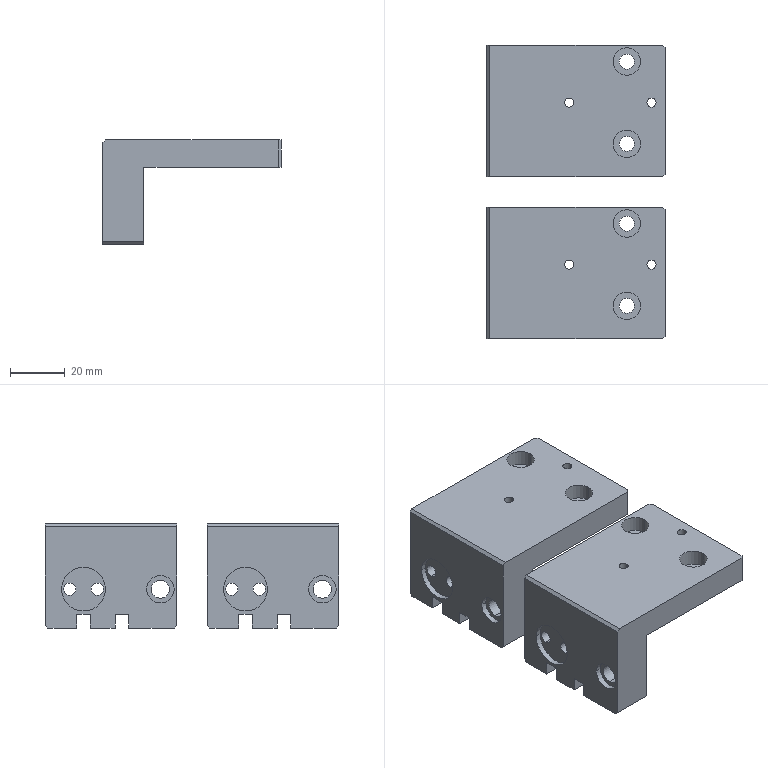NC program | NX | posted with a generic post | part box 65 x 107 x 38 mm
Whole program:
N10 G17 G21 G94 G90
(FLOOR_WALL_COPY , TOOL : D80)
N12 T19 M6
N14 G54
N16 G17 G0 G90 X96.5 Y0. B0. C0. S6500 M3
N18 G43 Z30. H19
N20 Z9.
N22 G94 G1 Z6. F1500.
N24 X93.5
N26 X-93.5
N28 X-96.5
N30 Z9.
N32 G0 Z30.
N34 X96.5
N36 Z8.
N38 G1 Z5.
N40 X93.5
N42 X-93.5
N44 X-96.5
N46 Z8.
N48 G0 Z30.
N50 X96.5
N52 Z7.
N54 G1 Z4.
N56 X93.5
N58 X-93.5
N60 X-96.5
N62 Z7.
N64 G0 Z30.
N66 X96.5
N68 Z6.
N70 G1 Z3.
N72 X93.5
N74 X-93.5
N76 X-96.5
N78 Z6.
N80 G0 Z30.
N82 X96.5
N84 Z5.
N86 G1 Z2.
N88 X93.5
N90 X-93.5
N92 X-96.5
N94 Z5.
N96 G0 Z30.
N98 X96.5
N100 Z4.
N102 G1 Z1.
N104 X93.5
N106 X-93.5
N108 X-96.5
N110 Z4.
N112 G0 Z30.
N114 X96.5
N116 Z3.
N118 G1 Z0.
N120 X93.5
N122 X-93.5
N124 X-96.5
N126 Z3.
N128 G0 Z30.
N130 M5
(FLOOR_WALL_1 , TOOL : D10)
N132 T15 M6
N134 G54
N136 G17 G0 G90 X-2.01 Y-39.324 B0. C0. S9500 M3
N138 G43 Z30. H15
N140 Z-5.925
N142 G94 G1 Z-8.925 F1000.
N144 X-3.063 Y-37.5
N146 G3 X-3.929 Y-37. R1.
N148 G1 X-55.071 F3500.
N150 X-55.57 Y-36.502
N152 X-3.43
N154 X-2.932 Y-36.003
N156 X-56.068
N158 X-56.567 Y-35.505
N160 X-2.433
N162 X-1.935 Y-35.006
N164 X-57.065
N166 X-57.563 Y-34.508
N168 X-1.437
N170 X-0.938 Y-34.009
N172 X-58.062
N174 X-58.5 Y-33.571
N176 Y-33.511
N178 X-0.5
N180 Y-33.012
N182 X-58.5
N184 Y-32.514
N186 X-0.5
N188 Y-32.015
N190 X-58.5
N192 Y-31.517
N194 X-0.5
N196 Y-31.018
N198 X-58.5
N200 Y-30.52
N202 X-0.5
N204 Y-30.021
N206 X-58.5
N208 Y-29.523
N210 X-0.5
N212 Y-29.024
N214 X-58.5
N216 Y-28.526
N218 X-0.5
N220 Y-28.027
N222 X-58.5
N224 Y-27.529
N226 X-0.5
N228 Y-27.03
N230 X-58.5
N232 Y-26.532
N234 X-0.5
N236 Y-26.033
N238 X-58.5
N240 Y-25.535
N242 X-0.5
N244 Y-25.036
N246 X-58.5
N248 Y-24.538
N250 X-0.5
N252 Y-24.039
N254 X-58.5
N256 Y-23.541
N258 X-0.5
N260 Y-23.042
N262 X-58.5
N264 Y-22.544
N266 X-0.5
N268 Y-22.045
N270 X-58.5
N272 Y-21.547
N274 X-0.5
N276 Y-21.048
N278 X-58.5
N280 Y-20.55
N282 X-0.5
N284 Y-20.052
N286 X-58.5
N288 Y-19.553
N290 X-0.5
N292 Y-19.055
N294 X-58.5
N296 Y-18.556
N298 X-0.5
N300 Y-18.058
N302 X-58.5
N304 Y-17.559
N306 X-0.5
N308 Y-17.061
N310 X-58.5
N312 Y-16.562
N314 X-0.5
N316 Y-16.064
N318 X-58.5
N320 Y-15.565
N322 X-0.5
N324 Y-15.067
N326 X-58.5
N328 Y-14.568
N330 X-0.5
N332 Y-14.07
N334 X-58.5
N336 Y-13.571
N338 X-0.5
N340 Y-13.073
N342 X-58.5
N344 Y-12.574
N346 X-0.5
N348 Y-12.076
N350 X-58.5
N352 Y-11.577
N354 X-0.5
N356 Y-11.079
N358 X-58.5
N360 Y-10.58
N362 X-0.5
N364 Y-10.082
N366 X-58.5
N368 Y-9.583
N370 X-0.5
N372 Y-9.085
N374 X-58.5
N376 Y-8.586
N378 X-0.5
N380 Y-8.088
N382 X-58.5
N384 Y-7.589
N386 X-0.5
N388 Y-7.091
N390 X-58.5
N392 Y-6.592
N394 X-0.5
N396 Y-6.094
N398 X-58.5
N400 Y-5.595
N402 X-0.5
N404 Y-5.097
N406 X-58.5
N408 Y-4.598
N410 X-0.5
N412 Y-4.1
N414 X-58.5
N416 Y-3.602
N418 X-0.5
N420 Y-3.103
N422 X-58.5
N424 Y-2.605
N426 X-0.5
N428 Y-2.106
N430 X-58.5
N432 Y-1.608
N434 X-0.5
N436 Y-1.109
N438 X-58.5
N440 Y-0.611
N442 X-0.5
N444 Y-0.112
N446 X-58.5
N448 Y0.386
N450 X-0.5
N452 Y0.885
N454 X-58.5
N456 Y1.383
N458 X-0.5
N460 Y1.882
N462 X-58.5
N464 Y2.38
N466 X-0.5
N468 Y2.879
N470 X-58.5
N472 Y3.377
N474 X-0.5
N476 Y3.876
N478 X-58.5
N480 Y4.374
N482 X-0.5
N484 Y4.873
N486 X-58.5
N488 Y5.371
N490 X-0.5
N492 Y5.87
N494 X-58.5
N496 Y6.368
N498 X-0.5
N500 Y6.867
N502 X-58.5
N504 Y7.365
N506 X-0.5
N508 Y7.864
N510 X-58.5
N512 Y8.362
N514 X-0.5
N516 Y8.861
N518 X-58.5
N520 Y9.359
N522 X-0.5
N524 Y9.858
N526 X-58.5
N528 Y10.356
N530 X-0.5
N532 Y10.855
N534 X-58.5
N536 Y11.353
N538 X-0.5
N540 Y11.852
N542 X-58.5
N544 Y12.35
N546 X-0.5
N548 Z-5.925
N550 G0 Z30.
N552 X-2.01 Y-39.324
N554 Z-24.85
N556 G1 Z-27.85 F1000.
N558 X-3.063 Y-37.5
N560 G3 X-3.929 Y-37. R1.
N562 G1 X-55.071 F3500.
N564 X-55.57 Y-36.502
N566 X-3.43
N568 X-2.932 Y-36.003
N570 X-56.068
N572 X-56.567 Y-35.505
N574 X-2.433
N576 X-1.935 Y-35.006
N578 X-57.065
N580 X-57.563 Y-34.508
N582 X-1.437
N584 X-0.938 Y-34.009
N586 X-58.062
N588 X-58.5 Y-33.571
N590 Y-33.511
N592 X-0.5
N594 Y-33.012
N596 X-58.5
N598 Y-32.514
N600 X-0.5
N602 Y-32.015
N604 X-58.5
N606 Y-31.517
N608 X-0.5
N610 Y-31.018
N612 X-58.5
N614 Y-30.52
N616 X-0.5
N618 Y-30.021
N620 X-58.5
N622 Y-29.523
N624 X-0.5
N626 Y-29.024
N628 X-58.5
N630 Y-28.526
N632 X-0.5
N634 Y-28.027
N636 X-58.5
N638 Y-27.529
N640 X-0.5
N642 Y-27.03
N644 X-58.5
N646 Y-26.532
N648 X-0.5
N650 Y-26.033
N652 X-58.5
N654 Y-25.535
N656 X-0.5
N658 Y-25.036
N660 X-58.5
N662 Y-24.538
N664 X-0.5
N666 Y-24.039
N668 X-58.5
N670 Y-23.541
N672 X-0.5
N674 Y-23.042
N676 X-58.5
N678 Y-22.544
N680 X-0.5
N682 Y-22.045
N684 X-58.5
N686 Y-21.547
N688 X-0.5
N690 Y-21.048
N692 X-58.5
N694 Y-20.55
N696 X-0.5
N698 Y-20.052
N700 X-58.5
N702 Y-19.553
N704 X-0.5
N706 Y-19.055
N708 X-58.5
N710 Y-18.556
N712 X-0.5
N714 Y-18.058
N716 X-58.5
N718 Y-17.559
N720 X-0.5
N722 Y-17.061
N724 X-58.5
N726 Y-16.562
N728 X-0.5
N730 Y-16.064
N732 X-58.5
N734 Y-15.565
N736 X-0.5
N738 Y-15.067
N740 X-58.5
N742 Y-14.568
N744 X-0.5
N746 Y-14.07
N748 X-58.5
N750 Y-13.571
N752 X-0.5
N754 Y-13.073
N756 X-58.5
N758 Y-12.574
N760 X-0.5
N762 Y-12.076
N764 X-58.5
N766 Y-11.577
N768 X-0.5
N770 Y-11.079
N772 X-58.5
N774 Y-10.58
N776 X-0.5
N778 Y-10.082
N780 X-58.5
N782 Y-9.583
N784 X-0.5
N786 Y-9.085
N788 X-58.5
N790 Y-8.586
N792 X-0.5
N794 Y-8.088
N796 X-58.5
N798 Y-7.589
N800 X-0.5
N802 Y-7.091
N804 X-58.5
N806 Y-6.592
N808 X-0.5
N810 Y-6.094
N812 X-58.5
N814 Y-5.595
N816 X-0.5
N818 Y-5.097
N820 X-58.5
N822 Y-4.598
N824 X-0.5
N826 Y-4.1
N828 X-58.5
N830 Y-3.602
N832 X-0.5
N834 Y-3.103
N836 X-58.5
N838 Y-2.605
N840 X-0.5
N842 Y-2.106
N844 X-58.5
N846 Y-1.608
N848 X-0.5
N850 Y-1.109
N852 X-58.5
N854 Y-0.611
N856 X-0.5
N858 Y-0.112
N860 X-58.5
N862 Y0.386
N864 X-0.5
N866 Y0.885
N868 X-58.5
N870 Y1.383
N872 X-0.5
N874 Y1.882
N876 X-58.5
N878 Y2.38
N880 X-0.5
N882 Y2.879
N884 X-58.5
N886 Y3.377
N888 X-0.5
N890 Y3.876
N892 X-58.5
N894 Y4.374
N896 X-0.5
N898 Y4.873
N900 X-58.5
N902 Y5.371
N904 X-0.5
N906 Y5.87
N908 X-58.5
N910 Y6.368
N912 X-0.5
N914 Y6.867
N916 X-58.5
N918 Y7.365
N920 X-0.5
N922 Y7.864
N924 X-58.5
N926 Y8.362
N928 X-0.5
N930 Y8.861
N932 X-58.5
N934 Y9.359
N936 X-0.5
N938 Y9.858
N940 X-58.5
N942 Y10.356
N944 X-0.5
N946 Y10.855
N948 X-58.5
N950 Y11.353
N952 X-0.5
N954 Y11.852
N956 X-58.5
N958 Y12.35
N960 X-0.5
N962 Z-24.85
N964 G0 Z30.
N966 X56.99 Y-39.324
N968 Z-5.925
N970 G1 Z-8.925 F1000.
N972 X55.937 Y-37.5
N974 G3 X55.071 Y-37. R1.
N976 G1 X3.929 F3500.
N978 X3.43 Y-36.502
N980 X55.57
N982 X56.068 Y-36.003
N984 X2.932
N986 X2.433 Y-35.505
N988 X56.567
N990 X57.065 Y-35.006
N992 X1.935
N994 X1.437 Y-34.508
N996 X57.563
N998 X58.062 Y-34.009
N1000 X0.938
N1002 X0.5 Y-33.571
N1004 Y-33.511
N1006 X58.5
N1008 Y-33.012
N1010 X0.5
N1012 Y-32.514
N1014 X58.5
N1016 Y-32.015
N1018 X0.5
N1020 Y-31.517
N1022 X58.5
N1024 Y-31.018
N1026 X0.5
N1028 Y-30.52
N1030 X58.5
N1032 Y-30.021
N1034 X0.5
N1036 Y-29.523
N1038 X58.5
N1040 Y-29.024
N1042 X0.5
N1044 Y-28.526
N1046 X58.5
N1048 Y-28.027
N1050 X0.5
N1052 Y-27.529
N1054 X58.5
N1056 Y-27.03
N1058 X0.5
N1060 Y-26.532
N1062 X58.5
N1064 Y-26.033
N1066 X0.5
N1068 Y-25.535
N1070 X58.5
N1072 Y-25.036
N1074 X0.5
N1076 Y-24.538
N1078 X58.5
N1080 Y-24.039
N1082 X0.5
N1084 Y-23.541
N1086 X58.5
N1088 Y-23.042
N1090 X0.5
N1092 Y-22.544
N1094 X58.5
N1096 Y-22.045
N1098 X0.5
N1100 Y-21.547
N1102 X58.5
N1104 Y-21.048
N1106 X0.5
N1108 Y-20.55
N1110 X58.5
N1112 Y-20.052
N1114 X0.5
N1116 Y-19.553
N1118 X58.5
N1120 Y-19.055
N1122 X0.5
N1124 Y-18.556
N1126 X58.5
N1128 Y-18.058
N1130 X0.5
N1132 Y-17.559
N1134 X58.5
N1136 Y-17.061
N1138 X0.5
N1140 Y-16.562
N1142 X58.5
N1144 Y-16.064
N1146 X0.5
N1148 Y-15.565
N1150 X58.5
N1152 Y-15.067
N1154 X0.5
N1156 Y-14.568
N1158 X58.5
N1160 Y-14.07
N1162 X0.5
N1164 Y-13.571
N1166 X58.5
N1168 Y-13.073
N1170 X0.5
N1172 Y-12.574
N1174 X58.5
N1176 Y-12.076
N1178 X0.5
N1180 Y-11.577
N1182 X58.5
N1184 Y-11.079
N1186 X0.5
N1188 Y-10.58
N1190 X58.5
N1192 Y-10.082
N1194 X0.5
N1196 Y-9.583
N1198 X58.5
N1200 Y-9.085
N1202 X0.5
N1204 Y-8.586
N1206 X58.5
N1208 Y-8.088
N1210 X0.5
N1212 Y-7.589
N1214 X58.5
N1216 Y-7.091
N1218 X0.5
N1220 Y-6.592
N1222 X58.5
N1224 Y-6.094
N1226 X0.5
N1228 Y-5.595
N1230 X58.5
N1232 Y-5.097
N1234 X0.5
N1236 Y-4.598
N1238 X58.5
N1240 Y-4.1
N1242 X0.5
N1244 Y-3.602
N1246 X58.5
N1248 Y-3.103
N1250 X0.5
N1252 Y-2.605
N1254 X58.5
N1256 Y-2.106
N1258 X0.5
N1260 Y-1.608
N1262 X58.5
N1264 Y-1.109
N1266 X0.5
N1268 Y-0.611
N1270 X58.5
N1272 Y-0.112
N1274 X0.5
N1276 Y0.386
N1278 X58.5
N1280 Y0.885
N1282 X0.5
N1284 Y1.383
N1286 X58.5
N1288 Y1.882
N1290 X0.5
N1292 Y2.38
N1294 X58.5
N1296 Y2.879
N1298 X0.5
N1300 Y3.377
N1302 X58.5
N1304 Y3.876
N1306 X0.5
N1308 Y4.374
N1310 X58.5
N1312 Y4.873
N1314 X0.5
N1316 Y5.371
N1318 X58.5
N1320 Y5.87
N1322 X0.5
N1324 Y6.368
N1326 X58.5
N1328 Y6.867
N1330 X0.5
N1332 Y7.365
N1334 X58.5
N1336 Y7.864
N1338 X0.5
N1340 Y8.362
N1342 X58.5
N1344 Y8.861
N1346 X0.5
N1348 Y9.359
N1350 X58.5
N1352 Y9.858
N1354 X0.5
N1356 Y10.356
N1358 X58.5
N1360 Y10.855
N1362 X0.5
N1364 Y11.353
N1366 X58.5
N1368 Y11.852
N1370 X0.5
N1372 Y12.35
N1374 X58.5
N1376 G2 X59.366 Y11.85 R1.
N1378 G1 X61.5 Y8.154
N1380 Z-5.925
N1382 G0 Z30.
N1384 X56.99 Y-39.324
N1386 Z-24.85
N1388 G1 Z-27.85 F1000.
N1390 X55.937 Y-37.5
N1392 G3 X55.071 Y-37. R1.
N1394 G1 X3.929 F3500.
N1396 X3.43 Y-36.502
N1398 X55.57
N1400 X56.068 Y-36.003
N1402 X2.932
N1404 X2.433 Y-35.505
N1406 X56.567
N1408 X57.065 Y-35.006
N1410 X1.935
N1412 X1.437 Y-34.508
N1414 X57.563
N1416 X58.062 Y-34.009
N1418 X0.938
N1420 X0.5 Y-33.571
N1422 Y-33.511
N1424 X58.5
N1426 Y-33.012
N1428 X0.5
N1430 Y-32.514
N1432 X58.5
N1434 Y-32.015
N1436 X0.5
N1438 Y-31.517
N1440 X58.5
N1442 Y-31.018
N1444 X0.5
N1446 Y-30.52
N1448 X58.5
N1450 Y-30.021
N1452 X0.5
N1454 Y-29.523
N1456 X58.5
N1458 Y-29.024
N1460 X0.5
N1462 Y-28.526
N1464 X58.5
N1466 Y-28.027
N1468 X0.5
N1470 Y-27.529
N1472 X58.5
N1474 Y-27.03
N1476 X0.5
N1478 Y-26.532
N1480 X58.5
N1482 Y-26.033
N1484 X0.5
N1486 Y-25.535
N1488 X58.5
N1490 Y-25.036
N1492 X0.5
N1494 Y-24.538
N1496 X58.5
N1498 Y-24.039
N1500 X0.5
N1502 Y-23.541
N1504 X58.5
N1506 Y-23.042
N1508 X0.5
N1510 Y-22.544
N1512 X58.5
N1514 Y-22.045
N1516 X0.5
N1518 Y-21.547
N1520 X58.5
N1522 Y-21.048
N1524 X0.5
N1526 Y-20.55
N1528 X58.5
N1530 Y-20.052
N1532 X0.5
N1534 Y-19.553
N1536 X58.5
N1538 Y-19.055
N1540 X0.5
N1542 Y-18.556
N1544 X58.5
N1546 Y-18.058
N1548 X0.5
N1550 Y-17.559
N1552 X58.5
N1554 Y-17.061
N1556 X0.5
N1558 Y-16.562
N1560 X58.5
N1562 Y-16.064
N1564 X0.5
N1566 Y-15.565
N1568 X58.5
N1570 Y-15.067
N1572 X0.5
N1574 Y-14.568
N1576 X58.5
N1578 Y-14.07
N1580 X0.5
N1582 Y-13.571
N1584 X58.5
N1586 Y-13.073
N1588 X0.5
N1590 Y-12.574
N1592 X58.5
N1594 Y-12.076
N1596 X0.5
N1598 Y-11.577
N1600 X58.5
N1602 Y-11.079
N1604 X0.5
N1606 Y-10.58
N1608 X58.5
N1610 Y-10.082
N1612 X0.5
N1614 Y-9.583
N1616 X58.5
N1618 Y-9.085
N1620 X0.5
N1622 Y-8.586
N1624 X58.5
N1626 Y-8.088
N1628 X0.5
N1630 Y-7.589
N1632 X58.5
N1634 Y-7.091
N1636 X0.5
N1638 Y-6.592
N1640 X58.5
N1642 Y-6.094
N1644 X0.5
N1646 Y-5.595
N1648 X58.5
N1650 Y-5.097
N1652 X0.5
N1654 Y-4.598
N1656 X58.5
N1658 Y-4.1
N1660 X0.5
N1662 Y-3.602
N1664 X58.5
N1666 Y-3.103
N1668 X0.5
N1670 Y-2.605
N1672 X58.5
N1674 Y-2.106
N1676 X0.5
N1678 Y-1.608
N1680 X58.5
N1682 Y-1.109
N1684 X0.5
N1686 Y-0.611
N1688 X58.5
N1690 Y-0.112
N1692 X0.5
N1694 Y0.386
N1696 X58.5
N1698 Y0.885
N1700 X0.5
N1702 Y1.383
N1704 X58.5
N1706 Y1.882
N1708 X0.5
N1710 Y2.38
N1712 X58.5
N1714 Y2.879
N1716 X0.5
N1718 Y3.377
N1720 X58.5
N1722 Y3.876
N1724 X0.5
N1726 Y4.374
N1728 X58.5
N1730 Y4.873
N1732 X0.5
N1734 Y5.371
N1736 X58.5
N1738 Y5.87
N1740 X0.5
N1742 Y6.368
N1744 X58.5
N1746 Y6.867
N1748 X0.5
N1750 Y7.365
N1752 X58.5
N1754 Y7.864
N1756 X0.5
N1758 Y8.362
N1760 X58.5
N1762 Y8.861
N1764 X0.5
N1766 Y9.359
N1768 X58.5
N1770 Y9.858
N1772 X0.5
N1774 Y10.356
N1776 X58.5
N1778 Y10.855
N1780 X0.5
N1782 Y11.353
N1784 X58.5
N1786 Y11.852
N1788 X0.5
N1790 Y12.35
N1792 X58.5
N1794 G2 X59.366 Y11.85 R1.
N1796 G1 X61.5 Y8.154
N1798 Z-24.85
N1800 G0 Z30.
N1802 M5
(FLOOR_WALL_2 , TOOL : D10JING)
N1804 T14 M6
N1806 G54
N1808 G17 G0 G90 X-61.65 Y11.847 B0. C0. S9500 M3
N1810 G43 Z30. H14
N1812 Z-25.
N1814 G94 G1 Z-28. F1500.
N1816 X-58.5
N1818 X-0.5
N1820 Y7.364
N1822 X-58.5
N1824 Y2.881
N1826 X-0.5
N1828 Y-1.602
N1830 X-58.5
N1832 Y-6.085
N1834 X-0.5
N1836 Y-10.568
N1838 X-58.5
N1840 Y-15.051
N1842 X-0.5
N1844 Y-19.534
N1846 X-58.5
N1848 Y-24.017
N1850 X-0.5
N1852 Y-28.5
N1854 X-58.5
N1856 X-61.5
N1858 Z-25.
N1860 G0 Z30.
N1862 X-0.5 Y-10.042
N1864 Z-22.
N1866 G1 Y12.35 Z-28.
N1868 X-58.5
N1870 X-61.65
N1872 Z-25.
N1874 G0 Z30.
N1876 X61.5 Y-32.497
N1878 Z-25.
N1880 G1 Z-28.
N1882 X58.5
N1884 X0.5
N1886 Y-27.57
N1888 X58.5
N1890 Y-22.642
N1892 X0.5
N1894 Y-17.715
N1896 X58.5
N1898 Y-12.787
N1900 X0.5
N1902 Y-7.86
N1904 X58.5
N1906 Y-2.932
N1908 X0.5
N1910 Y1.995
N1912 X58.5
N1914 Y6.923
N1916 X0.5
N1918 Y11.85
N1920 X58.5
N1922 X61.65
N1924 Z-25.
N1926 G0 Z30.
N1928 Y12.35
N1930 Z-25.
N1932 G1 Z-28.
N1934 X58.5
N1936 X0.5
N1938 X-2.5
N1940 Y9.35
N1942 Z-25.
N1944 G0 Z30.
(FLOOR_WALL_2_COPY , TOOL : D10JING)
N1946 X-3.191 Y9.5
N1948 Z-6.
N1950 G1 Z-9.
N1952 X-4.634 Y12.
N1954 G3 X-5.5 Y12.5 R1.
N1956 G1 X-53.5
N1958 G3 X-54.366 Y12. R1.
N1960 G1 X-55.809 Y9.5
N1962 Z-6.
N1964 G0 Z30.
N1966 X-3.191
N1968 Z-25.
N1970 G1 Z-28.
N1972 X-4.634 Y12.
N1974 G3 X-5.5 Y12.5 R1.
N1976 G1 X-53.5
N1978 G3 X-54.366 Y12. R1.
N1980 G1 X-55.809 Y9.5
N1982 Z-25.
N1984 G0 Z30.
N1986 X55.809
N1988 Z-6.
N1990 G1 Z-9.
N1992 X54.366 Y12.
N1994 G3 X53.5 Y12.5 R1.
N1996 G1 X5.5
N1998 G3 X4.634 Y12. R1.
N2000 G1 X3.191 Y9.5
N2002 Z-6.
N2004 G0 Z30.
N2006 X55.809
N2008 Z-25.
N2010 G1 Z-28.
N2012 X54.366 Y12.
N2014 G3 X53.5 Y12.5 R1.
N2016 G1 X5.5
N2018 G3 X4.634 Y12. R1.
N2020 G1 X3.191 Y9.5
N2022 Z-25.
N2024 G0 Z30.
N2026 M5
(FLOOR_WALL_3 , TOOL : D4)
N2028 T11 M6
N2030 G54
N2032 G17 G0 G90 X-39.5 Y37.5 B0. C0. S9500 M3
N2034 G43 Z30. H11
N2036 Z2.615
N2038 G94 G1 Z-0.385 F1500.
N2040 Y32.5
N2042 X-39.
N2044 Y17.5
N2046 X-40.
N2048 Y32.5
N2050 X-39.5
N2052 Y37.5
N2054 Z2.615
N2056 G0 Z2.231
N2058 G1 Z-0.769
N2060 Y32.5
N2062 X-39.
N2064 Y17.5
N2066 X-40.
N2068 Y32.5
N2070 X-39.5
N2072 Y37.5
N2074 Z2.231
N2076 G0 Z1.846
N2078 G1 Z-1.154
N2080 Y32.5
N2082 X-39.
N2084 Y17.5
N2086 X-40.
N2088 Y32.5
N2090 X-39.5
N2092 Y37.5
N2094 Z1.846
N2096 G0 Z1.462
N2098 G1 Z-1.538
N2100 Y32.5
N2102 X-39.
N2104 Y17.5
N2106 X-40.
N2108 Y32.5
N2110 X-39.5
N2112 Y37.5
N2114 Z1.462
N2116 G0 Z1.077
N2118 G1 Z-1.923
N2120 Y32.5
N2122 X-39.
N2124 Y17.5
N2126 X-40.
N2128 Y32.5
N2130 X-39.5
N2132 Y37.5
N2134 Z1.077
N2136 G0 Z0.692
N2138 G1 Z-2.308
N2140 Y32.5
N2142 X-39.
N2144 Y17.5
N2146 X-40.
N2148 Y32.5
N2150 X-39.5
N2152 Y37.5
N2154 Z0.692
N2156 G0 Z0.308
N2158 G1 Z-2.692
N2160 Y32.5
N2162 X-39.
N2164 Y17.5
N2166 X-40.
N2168 Y32.5
N2170 X-39.5
N2172 Y37.5
N2174 Z0.308
N2176 G0 Z-0.077
N2178 G1 Z-3.077
N2180 Y32.5
N2182 X-39.
N2184 Y17.5
N2186 X-40.
N2188 Y32.5
N2190 X-39.5
N2192 Y37.5
N2194 Z-0.077
N2196 G0 Z-0.462
N2198 G1 Z-3.462
N2200 Y32.5
N2202 X-39.
N2204 Y17.5
N2206 X-40.
N2208 Y32.5
N2210 X-39.5
N2212 Y37.5
N2214 Z-0.462
N2216 G0 Z-0.846
N2218 G1 Z-3.846
N2220 Y32.5
N2222 X-39.
N2224 Y17.5
N2226 X-40.
N2228 Y32.5
N2230 X-39.5
N2232 Y37.5
N2234 Z-0.846
N2236 G0 Z-1.231
N2238 G1 Z-4.231
N2240 Y32.5
N2242 X-39.
N2244 Y17.5
N2246 X-40.
N2248 Y32.5
N2250 X-39.5
N2252 Y37.5
N2254 Z-1.231
N2256 G0 Z-1.615
N2258 G1 Z-4.615
N2260 Y32.5
N2262 X-39.
N2264 Y17.5
N2266 X-40.
N2268 Y32.5
N2270 X-39.5
N2272 Y37.5
N2274 Z-1.615
N2276 G0 Z-2.
N2278 G1 Z-5.
N2280 Y32.5
N2282 X-39.
N2284 Y17.5
N2286 X-40.
N2288 Y32.5
N2290 X-39.5
N2292 Y37.5
N2294 Z-2.
N2296 G0 Z30.
N2298 X-25.5
N2300 Z2.615
N2302 G1 Z-0.385
N2304 Y32.5
N2306 X-25.
N2308 Y17.5
N2310 X-26.
N2312 Y32.5
N2314 X-25.5
N2316 Y37.5
N2318 Z2.615
N2320 G0 Z2.231
N2322 G1 Z-0.769
N2324 Y32.5
N2326 X-25.
N2328 Y17.5
N2330 X-26.
N2332 Y32.5
N2334 X-25.5
N2336 Y37.5
N2338 Z2.231
N2340 G0 Z1.846
N2342 G1 Z-1.154
N2344 Y32.5
N2346 X-25.
N2348 Y17.5
N2350 X-26.
N2352 Y32.5
N2354 X-25.5
N2356 Y37.5
N2358 Z1.846
N2360 G0 Z1.462
N2362 G1 Z-1.538
N2364 Y32.5
N2366 X-25.
N2368 Y17.5
N2370 X-26.
N2372 Y32.5
N2374 X-25.5
N2376 Y37.5
N2378 Z1.462
N2380 G0 Z1.077
N2382 G1 Z-1.923
N2384 Y32.5
N2386 X-25.
N2388 Y17.5
N2390 X-26.
N2392 Y32.5
N2394 X-25.5
N2396 Y37.5
N2398 Z1.077
N2400 G0 Z0.692
N2402 G1 Z-2.308
N2404 Y32.5
N2406 X-25.
N2408 Y17.5
N2410 X-26.
N2412 Y32.5
N2414 X-25.5
N2416 Y37.5
N2418 Z0.692
N2420 G0 Z0.308
N2422 G1 Z-2.692
N2424 Y32.5
N2426 X-25.
N2428 Y17.5
N2430 X-26.
N2432 Y32.5
N2434 X-25.5
N2436 Y37.5
N2438 Z0.308
N2440 G0 Z-0.077
N2442 G1 Z-3.077
N2444 Y32.5
N2446 X-25.
N2448 Y17.5
N2450 X-26.
N2452 Y32.5
N2454 X-25.5
N2456 Y37.5
N2458 Z-0.077
N2460 G0 Z-0.462
N2462 G1 Z-3.462
N2464 Y32.5
N2466 X-25.
N2468 Y17.5
N2470 X-26.
N2472 Y32.5
N2474 X-25.5
N2476 Y37.5
N2478 Z-0.462
N2480 G0 Z-0.846
N2482 G1 Z-3.846
N2484 Y32.5
N2486 X-25.
N2488 Y17.5
N2490 X-26.
N2492 Y32.5
N2494 X-25.5
N2496 Y37.5
N2498 Z-0.846
N2500 G0 Z-1.231
N2502 G1 Z-4.231
N2504 Y32.5
N2506 X-25.
N2508 Y17.5
N2510 X-26.
N2512 Y32.5
N2514 X-25.5
N2516 Y37.5
N2518 Z-1.231
N2520 G0 Z-1.615
N2522 G1 Z-4.615
N2524 Y32.5
N2526 X-25.
N2528 Y17.5
N2530 X-26.
N2532 Y32.5
N2534 X-25.5
N2536 Y37.5
N2538 Z-1.615
N2540 G0 Z-2.
N2542 G1 Z-5.
N2544 Y32.5
N2546 X-25.
N2548 Y17.5
N2550 X-26.
N2552 Y32.5
N2554 X-25.5
N2556 Y37.5
N2558 Z-2.
N2560 G0 Z30.
N2562 X19.5
N2564 Z2.615
N2566 G1 Z-0.385
N2568 Y32.5
N2570 X20.
N2572 Y17.5
N2574 X19.
N2576 Y32.5
N2578 X19.5
N2580 Y37.5
N2582 Z2.615
N2584 G0 Z2.231
N2586 G1 Z-0.769
N2588 Y32.5
N2590 X20.
N2592 Y17.5
N2594 X19.
N2596 Y32.5
N2598 X19.5
N2600 Y37.5
N2602 Z2.231
N2604 G0 Z1.846
N2606 G1 Z-1.154
N2608 Y32.5
N2610 X20.
N2612 Y17.5
N2614 X19.
N2616 Y32.5
N2618 X19.5
N2620 Y37.5
N2622 Z1.846
N2624 G0 Z1.462
N2626 G1 Z-1.538
N2628 Y32.5
N2630 X20.
N2632 Y17.5
N2634 X19.
N2636 Y32.5
N2638 X19.5
N2640 Y37.5
N2642 Z1.462
N2644 G0 Z1.077
N2646 G1 Z-1.923
N2648 Y32.5
N2650 X20.
N2652 Y17.5
N2654 X19.
N2656 Y32.5
N2658 X19.5
N2660 Y37.5
N2662 Z1.077
N2664 G0 Z0.692
N2666 G1 Z-2.308
N2668 Y32.5
N2670 X20.
N2672 Y17.5
N2674 X19.
N2676 Y32.5
N2678 X19.5
N2680 Y37.5
N2682 Z0.692
N2684 G0 Z0.308
N2686 G1 Z-2.692
N2688 Y32.5
N2690 X20.
N2692 Y17.5
N2694 X19.
N2696 Y32.5
N2698 X19.5
N2700 Y37.5
N2702 Z0.308
N2704 G0 Z-0.077
N2706 G1 Z-3.077
N2708 Y32.5
N2710 X20.
N2712 Y17.5
N2714 X19.
N2716 Y32.5
N2718 X19.5
N2720 Y37.5
N2722 Z-0.077
N2724 G0 Z-0.462
N2726 G1 Z-3.462
N2728 Y32.5
N2730 X20.
N2732 Y17.5
N2734 X19.
N2736 Y32.5
N2738 X19.5
N2740 Y37.5
N2742 Z-0.462
N2744 G0 Z-0.846
N2746 G1 Z-3.846
N2748 Y32.5
N2750 X20.
N2752 Y17.5
N2754 X19.
N2756 Y32.5
N2758 X19.5
N2760 Y37.5
N2762 Z-0.846
N2764 G0 Z-1.231
N2766 G1 Z-4.231
N2768 Y32.5
N2770 X20.
N2772 Y17.5
N2774 X19.
N2776 Y32.5
N2778 X19.5
N2780 Y37.5
N2782 Z-1.231
N2784 G0 Z-1.615
N2786 G1 Z-4.615
N2788 Y32.5
N2790 X20.
N2792 Y17.5
N2794 X19.
N2796 Y32.5
N2798 X19.5
N2800 Y37.5
N2802 Z-1.615
N2804 G0 Z-2.
N2806 G1 Z-5.
N2808 Y32.5
N2810 X20.
N2812 Y17.5
N2814 X19.
N2816 Y32.5
N2818 X19.5
N2820 Y37.5
N2822 Z-2.
N2824 G0 Z30.
N2826 X33.5
N2828 Z2.615
N2830 G1 Z-0.385
N2832 Y32.5
N2834 X34.
N2836 Y17.5
N2838 X33.
N2840 Y32.5
N2842 X33.5
N2844 Y37.5
N2846 Z2.615
N2848 G0 Z2.231
N2850 G1 Z-0.769
N2852 Y32.5
N2854 X34.
N2856 Y17.5
N2858 X33.
N2860 Y32.5
N2862 X33.5
N2864 Y37.5
N2866 Z2.231
N2868 G0 Z1.846
N2870 G1 Z-1.154
N2872 Y32.5
N2874 X34.
N2876 Y17.5
N2878 X33.
N2880 Y32.5
N2882 X33.5
N2884 Y37.5
N2886 Z1.846
N2888 G0 Z1.462
N2890 G1 Z-1.538
N2892 Y32.5
N2894 X34.
N2896 Y17.5
N2898 X33.
N2900 Y32.5
N2902 X33.5
N2904 Y37.5
N2906 Z1.462
N2908 G0 Z1.077
N2910 G1 Z-1.923
N2912 Y32.5
N2914 X34.
N2916 Y17.5
N2918 X33.
N2920 Y32.5
N2922 X33.5
N2924 Y37.5
N2926 Z1.077
N2928 G0 Z0.692
N2930 G1 Z-2.308
N2932 Y32.5
N2934 X34.
N2936 Y17.5
N2938 X33.
N2940 Y32.5
N2942 X33.5
N2944 Y37.5
N2946 Z0.692
N2948 G0 Z0.308
N2950 G1 Z-2.692
N2952 Y32.5
N2954 X34.
N2956 Y17.5
N2958 X33.
N2960 Y32.5
N2962 X33.5
N2964 Y37.5
N2966 Z0.308
N2968 G0 Z-0.077
N2970 G1 Z-3.077
N2972 Y32.5
N2974 X34.
N2976 Y17.5
N2978 X33.
N2980 Y32.5
N2982 X33.5
N2984 Y37.5
N2986 Z-0.077
N2988 G0 Z-0.462
N2990 G1 Z-3.462
N2992 Y32.5
N2994 X34.
N2996 Y17.5
N2998 X33.
N3000 Y32.5
N3002 X33.5
N3004 Y37.5
N3006 Z-0.462
N3008 G0 Z-0.846
N3010 G1 Z-3.846
N3012 Y32.5
N3014 X34.
N3016 Y17.5
N3018 X33.
N3020 Y32.5
N3022 X33.5
N3024 Y37.5
N3026 Z-0.846
N3028 G0 Z-1.231
N3030 G1 Z-4.231
N3032 Y32.5
N3034 X34.
N3036 Y17.5
N3038 X33.
N3040 Y32.5
N3042 X33.5
N3044 Y37.5
N3046 Z-1.231
N3048 G0 Z-1.615
N3050 G1 Z-4.615
N3052 Y32.5
N3054 X34.
N3056 Y17.5
N3058 X33.
N3060 Y32.5
N3062 X33.5
N3064 Y37.5
N3066 Z-1.615
N3068 G0 Z-2.
N3070 G1 Z-5.
N3072 Y32.5
N3074 X34.
N3076 Y17.5
N3078 X33.
N3080 Y32.5
N3082 X33.5
N3084 Y37.5
N3086 Z-2.
N3088 G0 Z30.
N3090 M5
(PLANAR_MILL_COPY_COPY_COPY_COPY , TOOL : D6A45)
N3092 T01 M6
N3094 G54
N3096 G17 G0 G90 X45.616 Y16.1 B0. C0. S9500 M3
N3098 G43 Z30. H1
N3100 Z0.5
N3102 G94 G1 Z-1. F1250.
N3104 G3 X44.75 Y16.6 R1.
N3106 G1 X36.
N3108 G2 X35.1 Y17.5 R0.9
N3110 G1 Y32.5
N3112 G2 X36. Y33.4 R0.9
N3114 G1 X53.5
N3116 G2 X54.4 Y32.5 R0.9
N3118 G1 Y17.5
N3120 G2 X53.5 Y16.6 R0.9
N3122 G1 X44.75
N3124 G3 X43.884 Y16.1 R1.
N3126 G1 Z0.5
N3128 G0 Z30.
N3130 X32.4 Y25.866
N3132 Z0.5
N3134 G1 Z-1.
N3136 G3 X31.9 Y25. R1.
N3138 G1 Y17.5
N3140 G2 X31. Y16.6 R0.9
N3142 G1 X22.
N3144 G2 X21.1 Y17.5 R0.9
N3146 G1 Y32.5
N3148 G2 X22. Y33.4 R0.9
N3150 G1 X31.
N3152 G2 X31.9 Y32.5 R0.9
N3154 G1 Y25.
N3156 G3 X32.4 Y24.134 R1.
N3158 G1 Z0.5
N3160 G0 Z30.
N3162 X18.4 Y25.866
N3164 Z0.5
N3166 G1 Z-1.
N3168 G3 X17.9 Y25. R1.
N3170 G1 Y17.5
N3172 G2 X17. Y16.6 R0.9
N3174 G1 X5.5
N3176 G2 X4.6 Y17.5 R0.9
N3178 G1 Y32.5
N3180 G2 X5.5 Y33.4 R0.9
N3182 G1 X17.
N3184 G2 X17.9 Y32.5 R0.9
N3186 G1 Y25.
N3188 G3 X18.4 Y24.134 R1.
N3190 G1 Z0.5
N3192 G0 Z30.
N3194 X-13.384 Y16.1
N3196 Z0.5
N3198 G1 Z-1.
N3200 G3 X-14.25 Y16.6 R1.
N3202 G1 X-23.
N3204 G2 X-23.9 Y17.5 R0.9
N3206 G1 Y32.5
N3208 G2 X-23. Y33.4 R0.9
N3210 G1 X-5.5
N3212 G2 X-4.6 Y32.5 R0.9
N3214 G1 Y17.5
N3216 G2 X-5.5 Y16.6 R0.9
N3218 G1 X-14.25
N3220 G3 X-15.116 Y16.1 R1.
N3222 G1 Z0.5
N3224 G0 Z30.
N3226 X-26.6 Y25.866
N3228 Z0.5
N3230 G1 Z-1.
N3232 G3 X-27.1 Y25. R1.
N3234 G1 Y17.5
N3236 G2 X-28. Y16.6 R0.9
N3238 G1 X-37.
N3240 G2 X-37.9 Y17.5 R0.9
N3242 G1 Y32.5
N3244 G2 X-37. Y33.4 R0.9
N3246 G1 X-28.
N3248 G2 X-27.1 Y32.5 R0.9
N3250 G1 Y25.
N3252 G3 X-26.6 Y24.134 R1.
N3254 G1 Z0.5
N3256 G0 Z30.
N3258 X-54.9
N3260 Z0.5
N3262 G1 Z-1.
N3264 G3 X-54.4 Y25. R1.
N3266 G1 Y32.5
N3268 G2 X-53.5 Y33.4 R0.9
N3270 G1 X-42.
N3272 G2 X-41.1 Y32.5 R0.9
N3274 G1 Y17.5
N3276 G2 X-42. Y16.6 R0.9
N3278 G1 X-53.5
N3280 G2 X-54.4 Y17.5 R0.9
N3282 G1 Y25.
N3284 G3 X-54.9 Y25.866 R1.
N3286 G1 Z0.5
N3288 G0 Z30.
(PLANAR_MILL_COPY_COPY_COPY_COPY_COPY , TOOL : D6A45)
N3290 X49.825 Y10.563
N3292 Z-27.5
N3294 G1 X49.759 Y10.6 Z-27.52
N3296 X49.5 Z-27.59
N3298 X49.241 Z-27.659
N3300 X48.701 Y10.299 Z-27.825
N3302 X48.4 Y9.759 Z-27.991
N3304 Y9.241 Z-28.129
N3306 X48.701 Y8.701 Z-28.295
N3308 X49.241 Y8.4 Z-28.461
N3310 X49.759 Z-28.599
N3312 X50.299 Y8.701 Z-28.765
N3314 X50.6 Y9.241 Z-28.931
N3316 Y9.5 Z-29.
N3318 G3 X49.5 Y10.6 R1.1
N3320 X50.6 Y9.5 R-1.1
N3322 X50.1 Y10.366 R1.
N3324 G1 Z-27.5
N3326 G0 Z30.
N3328 X26.924 Y1.874
N3330 Z-27.5
N3332 G1 X27.052 Y1.948 Z-27.54
N3334 X27.25 Y2.286 Z-27.644
N3336 Y2.714 Z-27.759
N3338 X27.052 Y3.052 Z-27.864
N3340 X26.714 Y3.25 Z-27.969
N3342 X26.286 Z-28.084
N3344 X25.948 Y3.052 Z-28.189
N3346 X25.75 Y2.714 Z-28.294
N3348 Y2.286 Z-28.408
N3350 X25.948 Y1.948 Z-28.513
N3352 X26.286 Y1.75 Z-28.618
N3354 X26.714 Z-28.733
N3356 X27.052 Y1.948 Z-28.838
N3358 X27.25 Y2.286 Z-28.943
N3360 Y2.5 Z-29.
N3362 G3 X26.5 Y3.25 R0.75
N3364 X27.25 Y2.5 R-0.75
N3366 X27. Y2.933 R0.5
N3368 G1 Z-27.5
N3370 G0 Z30.
N3372 X55.813 Y13.408
N3374 Z-27.5
N3376 G1 Z-29.
N3378 X55.365 Y13.857
N3380 G3 X54.4 Y14.118 R1.
N3382 G1 Y-31.459
N3384 G2 X54.107 Y-32.166 R1.
N3386 G1 X53.166 Y-33.107
N3388 G2 X52.459 Y-33.4 R1.
N3390 G1 X6.541
N3392 G2 X5.834 Y-33.107 R1.
N3394 G1 X4.893 Y-32.166
N3396 G2 X4.6 Y-31.459 R1.
N3398 G1 Y14.118
N3400 G3 X3.635 Y13.857 R1.
N3402 G1 X3.187 Y13.408
N3404 Z-27.5
N3406 G0 Z30.
N3408 X-3.187
N3410 Z-27.5
N3412 G1 Z-29.
N3414 X-3.635 Y13.857
N3416 G3 X-4.6 Y14.118 R1.
N3418 G1 Y-31.459
N3420 G2 X-4.893 Y-32.166 R1.
N3422 G1 X-5.834 Y-33.107
N3424 G2 X-6.541 Y-33.4 R1.
N3426 G1 X-52.459
N3428 G2 X-53.166 Y-33.107 R1.
N3430 G1 X-54.107 Y-32.166
N3432 G2 X-54.4 Y-31.459 R1.
N3434 G1 Y14.118
N3436 G3 X-55.365 Y13.857 R1.
N3438 G1 X-55.813 Y13.408
N3440 Z-27.5
N3442 G0 Z30.
N3444 X-10.563 Y9.825
N3446 Z-27.5
N3448 G1 X-10.6 Y9.759 Z-27.52
N3450 Y9.5 Z-27.59
N3452 Y9.241 Z-27.659
N3454 X-10.299 Y8.701 Z-27.825
N3456 X-9.759 Y8.4 Z-27.991
N3458 X-9.241 Z-28.129
N3460 X-8.701 Y8.701 Z-28.295
N3462 X-8.4 Y9.241 Z-28.461
N3464 Y9.759 Z-28.599
N3466 X-8.701 Y10.299 Z-28.765
N3468 X-9.241 Y10.6 Z-28.931
N3470 X-9.5 Z-29.
N3472 G3 X-10.6 Y9.5 R1.1
N3474 X-9.5 Y10.6 R-1.1
N3476 X-10.366 Y10.1 R1.
N3478 G1 Z-27.5
N3480 G0 Z30.
N3482 X-32.924 Y3.126
N3484 Z-27.5
N3486 G1 X-33.052 Y3.052 Z-27.54
N3488 X-33.25 Y2.714 Z-27.644
N3490 Y2.286 Z-27.759
N3492 X-33.052 Y1.948 Z-27.864
N3494 X-32.714 Y1.75 Z-27.969
N3496 X-32.286 Z-28.084
N3498 X-31.948 Y1.948 Z-28.189
N3500 X-31.75 Y2.286 Z-28.294
N3502 Y2.714 Z-28.408
N3504 X-31.948 Y3.052 Z-28.513
N3506 X-32.286 Y3.25 Z-28.618
N3508 X-32.714 Z-28.733
N3510 X-33.052 Y3.052 Z-28.838
N3512 X-33.25 Y2.714 Z-28.943
N3514 Y2.5 Z-29.
N3516 G3 X-32.5 Y1.75 R0.75
N3518 X-33.25 Y2.5 R-0.75
N3520 X-33. Y2.067 R0.5
N3522 G1 Z-27.5
N3524 G0 Z30.
N3526 X-48.047 Y-18.149
N3528 Z-27.5
N3530 G1 Z-29.
N3532 X-48.85 Y-17.634
N3534 G3 X-49.35 Y-18.5 R1.
N3536 X-47.5 Y-20.35 R1.85
N3538 X-49.35 Y-18.5 R-1.85
N3540 X-48.85 Y-19.366 R1.
N3542 G1 X-48.047 Y-18.851
N3544 Z-27.5
N3546 G0 Z30.
N3548 X-33.126 Y-27.924
N3550 Z-27.5
N3552 G1 X-33.052 Y-28.052 Z-27.54
N3554 X-32.714 Y-28.25 Z-27.644
N3556 X-32.286 Z-27.759
N3558 X-31.948 Y-28.052 Z-27.864
N3560 X-31.75 Y-27.714 Z-27.969
N3562 Y-27.286 Z-28.084
N3564 X-31.948 Y-26.948 Z-28.189
N3566 X-32.286 Y-26.75 Z-28.294
N3568 X-32.714 Z-28.408
N3570 X-33.052 Y-26.948 Z-28.513
N3572 X-33.25 Y-27.286 Z-28.618
N3574 Y-27.714 Z-28.733
N3576 X-33.052 Y-28.052 Z-28.838
N3578 X-32.714 Y-28.25 Z-28.943
N3580 X-32.5 Z-29.
N3582 G3 X-31.75 Y-27.5 R0.75
N3584 X-32.5 Y-28.25 R-0.75
N3586 X-32.067 Y-28. R0.5
N3588 G1 Z-27.5
N3590 G0 Z30.
N3592 X-17.851 Y-19.047
N3594 Z-27.5
N3596 G1 Z-29.
N3598 X-18.366 Y-19.85
N3600 G3 X-17.5 Y-20.35 R1.
N3602 X-15.65 Y-18.5 R1.85
N3604 X-17.5 Y-20.35 R-1.85
N3606 X-16.634 Y-19.85 R1.
N3608 G1 X-17.149 Y-19.047
N3610 Z-27.5
N3612 G0 Z30.
N3614 X-8.437 Y-26.825
N3616 Z-27.5
N3618 G1 X-8.4 Y-26.759 Z-27.52
N3620 Y-26.5 Z-27.59
N3622 Y-26.241 Z-27.659
N3624 X-8.701 Y-25.701 Z-27.825
N3626 X-9.241 Y-25.4 Z-27.991
N3628 X-9.759 Z-28.129
N3630 X-10.299 Y-25.701 Z-28.295
N3632 X-10.6 Y-26.241 Z-28.461
N3634 Y-26.759 Z-28.599
N3636 X-10.299 Y-27.299 Z-28.765
N3638 X-9.759 Y-27.6 Z-28.931
N3640 X-9.5 Z-29.
N3642 G3 X-8.4 Y-26.5 R1.1
N3644 X-9.5 Y-27.6 R-1.1
N3646 X-8.634 Y-27.1 R1.
N3648 G1 Z-27.5
N3650 G0 Z30.
N3652 X11.149 Y-19.047
N3654 Z-27.5
N3656 G1 Z-29.
N3658 X10.634 Y-19.85
N3660 G3 X11.5 Y-20.35 R1.
N3662 X13.35 Y-18.5 R1.85
N3664 X11.5 Y-20.35 R-1.85
N3666 X12.366 Y-19.85 R1.
N3668 G1 X11.851 Y-19.047
N3670 Z-27.5
N3672 G0 Z30.
N3674 X25.874 Y-27.924
N3676 Z-27.5
N3678 G1 X25.948 Y-28.052 Z-27.54
N3680 X26.286 Y-28.25 Z-27.644
N3682 X26.714 Z-27.759
N3684 X27.052 Y-28.052 Z-27.864
N3686 X27.25 Y-27.714 Z-27.969
N3688 Y-27.286 Z-28.084
N3690 X27.052 Y-26.948 Z-28.189
N3692 X26.714 Y-26.75 Z-28.294
N3694 X26.286 Z-28.408
N3696 X25.948 Y-26.948 Z-28.513
N3698 X25.75 Y-27.286 Z-28.618
N3700 Y-27.714 Z-28.733
N3702 X25.948 Y-28.052 Z-28.838
N3704 X26.286 Y-28.25 Z-28.943
N3706 X26.5 Z-29.
N3708 G3 X27.25 Y-27.5 R0.75
N3710 X26.5 Y-28.25 R-0.75
N3712 X26.933 Y-28. R0.5
N3714 G1 Z-27.5
N3716 G0 Z30.
N3718 X42.047 Y-18.851
N3720 Z-27.5
N3722 G1 Z-29.
N3724 X42.85 Y-19.366
N3726 G3 X43.35 Y-18.5 R1.
N3728 X41.5 Y-16.65 R1.85
N3730 X43.35 Y-18.5 R-1.85
N3732 X42.85 Y-17.634 R1.
N3734 G1 X42.047 Y-18.149
N3736 Z-27.5
N3738 G0 Z30.
N3740 X49.825 Y-25.437
N3742 Z-27.5
N3744 G1 X49.759 Y-25.4 Z-27.52
N3746 X49.5 Z-27.59
N3748 X49.241 Z-27.659
N3750 X48.701 Y-25.701 Z-27.825
N3752 X48.4 Y-26.241 Z-27.991
N3754 Y-26.759 Z-28.129
N3756 X48.701 Y-27.299 Z-28.295
N3758 X49.241 Y-27.6 Z-28.461
N3760 X49.759 Z-28.599
N3762 X50.299 Y-27.299 Z-28.765
N3764 X50.6 Y-26.759 Z-28.931
N3766 Y-26.5 Z-29.
N3768 G3 X49.5 Y-25.4 R1.1
N3770 X50.6 Y-26.5 R-1.1
N3772 X50.1 Y-25.634 R1.
N3774 G1 Z-27.5
N3776 G0 Z30.
N3778 M5
N3780 M2